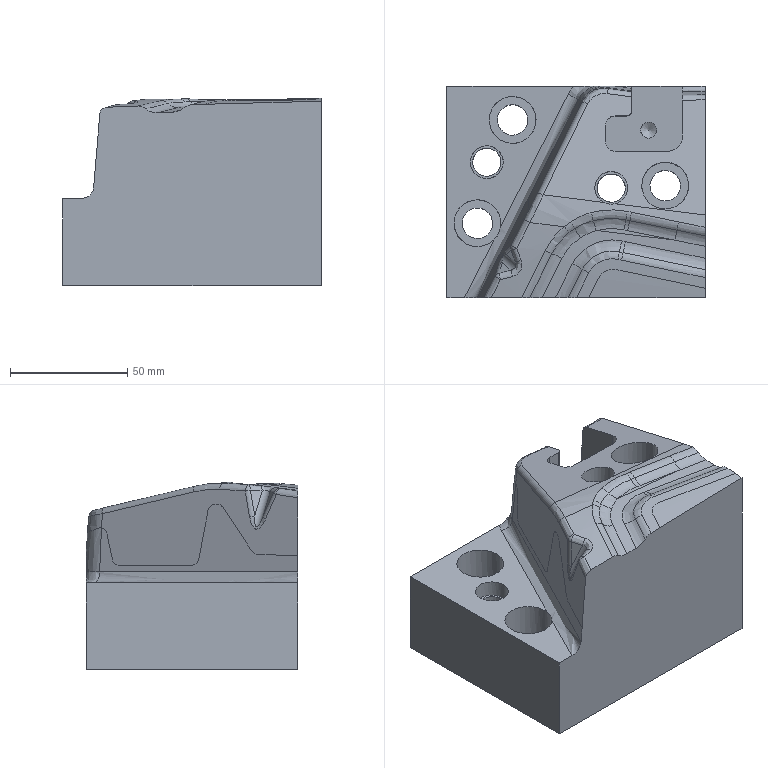Part | STEP file | gslz 2016.10.28-13_id1638_x_t | 1 solid | 93 faces | box 110 x 90.115 x 79.8 mm | volume 541473 mm3 | spline 52 | plane 19 | cylinder 19 | sphere 2 | cone 1 | commonest cylinder face diameters 5.5 x4 12 x3 13 x3 20 x3 8 x2 14 x2